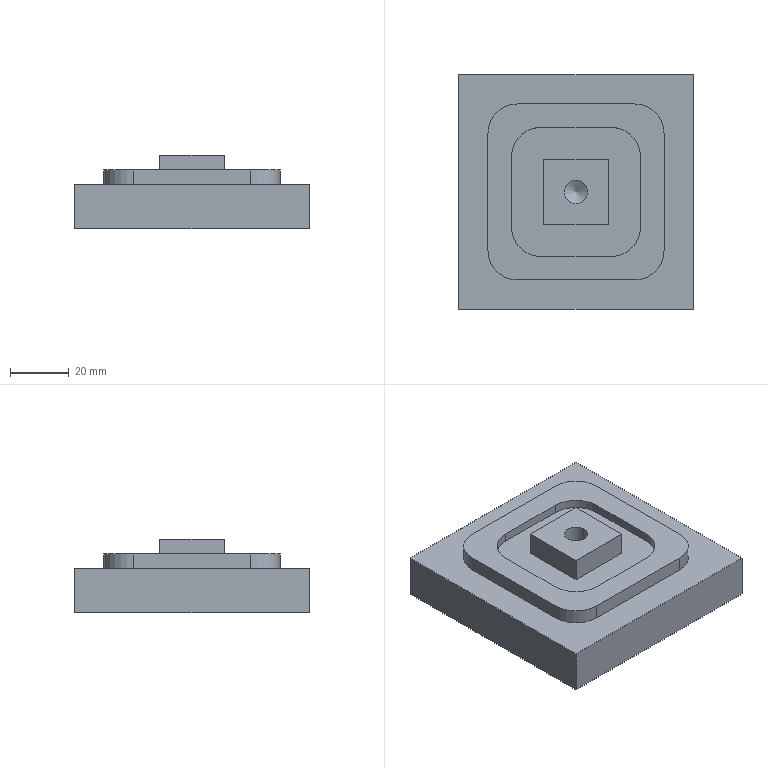NC program | NX | posted with a generic post | part box 80 x 80 x 25 mm
Whole program:
N10 G17 G21 G94 G90
(PLANAR_MILL , TOOL : T1D12)
N12 T01 M6
N14 G53
N16 G17 G0 G90 X32.505 Y-52. S2000 M3
N18 G43 Z10. H1
N20 Z2.
N22 G94 G1 Z-1. F1500.
N24 Y-40.
N26 X-40.
N28 Y-32.21
N30 X-32.8
N32 G3 X-32.21 Y-32.8 R17.69
N34 G1 X-32.8
N36 Y-32.21
N38 X-40.
N40 Y40.
N42 X-32.21
N44 Y32.8
N46 G3 X-32.8 Y32.21 R17.69
N48 G1 Y32.8
N50 X-32.21
N52 Y40.
N54 X40.
N56 Y32.21
N58 X32.8
N60 G3 X32.21 Y32.8 R17.69
N62 G1 X32.8
N64 Y32.21
N66 X40.
N68 Y-40.
N70 X32.505
N72 Y-32.8
N74 X32.21
N76 G3 X32.8 Y-32.21 R17.69
N78 G1 X31.758 Y-31.217
N80 G2 X20. Y-36.25 R16.25
N82 G1 X-20.
N84 G2 X-36.25 Y-20. R16.25
N86 G1 Y20.
N88 G2 X-20. Y36.25 R16.25
N90 G1 X20.
N92 G2 X36.25 Y20. R16.25
N94 G1 Y-20.
N96 G2 X31.758 Y-31.217 R16.25
N98 G1 X32.8 Y-32.21
N100 Y-32.8
N102 X32.505
N104 Y-52.
N106 Z2.
N108 G0 Z1.
N110 G1 Z-2.
N112 Y-40.
N114 X-40.
N116 Y-32.21
N118 X-32.8
N120 G3 X-32.21 Y-32.8 R17.69
N122 G1 X-32.8
N124 Y-32.21
N126 X-40.
N128 Y40.
N130 X-32.21
N132 Y32.8
N134 G3 X-32.8 Y32.21 R17.69
N136 G1 Y32.8
N138 X-32.21
N140 Y40.
N142 X40.
N144 Y32.21
N146 X32.8
N148 G3 X32.21 Y32.8 R17.69
N150 G1 X32.8
N152 Y32.21
N154 X40.
N156 Y-40.
N158 X32.505
N160 Y-32.8
N162 X32.21
N164 G3 X32.8 Y-32.21 R17.69
N166 G1 X31.758 Y-31.217
N168 G2 X20. Y-36.25 R16.25
N170 G1 X-20.
N172 G2 X-36.25 Y-20. R16.25
N174 G1 Y20.
N176 G2 X-20. Y36.25 R16.25
N178 G1 X20.
N180 G2 X36.25 Y20. R16.25
N182 G1 Y-20.
N184 G2 X31.758 Y-31.217 R16.25
N186 G1 X32.8 Y-32.21
N188 Y-32.8
N190 X32.505
N192 Y-52.
N194 Z1.
N196 G0 Z0.
N198 G1 Z-3.
N200 Y-40.
N202 X-40.
N204 Y-32.21
N206 X-32.8
N208 G3 X-32.21 Y-32.8 R17.69
N210 G1 X-32.8
N212 Y-32.21
N214 X-40.
N216 Y40.
N218 X-32.21
N220 Y32.8
N222 G3 X-32.8 Y32.21 R17.69
N224 G1 Y32.8
N226 X-32.21
N228 Y40.
N230 X40.
N232 Y32.21
N234 X32.8
N236 G3 X32.21 Y32.8 R17.69
N238 G1 X32.8
N240 Y32.21
N242 X40.
N244 Y-40.
N246 X32.505
N248 Y-32.8
N250 X32.21
N252 G3 X32.8 Y-32.21 R17.69
N254 G1 X31.758 Y-31.217
N256 G2 X20. Y-36.25 R16.25
N258 G1 X-20.
N260 G2 X-36.25 Y-20. R16.25
N262 G1 Y20.
N264 G2 X-20. Y36.25 R16.25
N266 G1 X20.
N268 G2 X36.25 Y20. R16.25
N270 G1 Y-20.
N272 G2 X31.758 Y-31.217 R16.25
N274 G1 X32.8 Y-32.21
N276 Y-32.8
N278 X32.505
N280 Y-52.
N282 Z0.
N284 G0 Z-1.
N286 G1 Z-4.
N288 Y-40.
N290 X-40.
N292 Y-32.21
N294 X-32.8
N296 G3 X-32.21 Y-32.8 R17.69
N298 G1 X-32.8
N300 Y-32.21
N302 X-40.
N304 Y40.
N306 X-32.21
N308 Y32.8
N310 G3 X-32.8 Y32.21 R17.69
N312 G1 Y32.8
N314 X-32.21
N316 Y40.
N318 X40.
N320 Y32.21
N322 X32.8
N324 G3 X32.21 Y32.8 R17.69
N326 G1 X32.8
N328 Y32.21
N330 X40.
N332 Y-40.
N334 X32.505
N336 Y-32.8
N338 X32.21
N340 G3 X32.8 Y-32.21 R17.69
N342 G1 X31.758 Y-31.217
N344 G2 X20. Y-36.25 R16.25
N346 G1 X-20.
N348 G2 X-36.25 Y-20. R16.25
N350 G1 Y20.
N352 G2 X-20. Y36.25 R16.25
N354 G1 X20.
N356 G2 X36.25 Y20. R16.25
N358 G1 Y-20.
N360 G2 X31.758 Y-31.217 R16.25
N362 G1 X32.8 Y-32.21
N364 Y-32.8
N366 X32.505
N368 Y-52.
N370 Z-1.
N372 G0 Z-2.
N374 G1 Z-5.
N376 Y-40.
N378 X-40.
N380 Y-32.21
N382 X-32.8
N384 G3 X-32.21 Y-32.8 R17.69
N386 G1 X-32.8
N388 Y-32.21
N390 X-40.
N392 Y40.
N394 X-32.21
N396 Y32.8
N398 G3 X-32.8 Y32.21 R17.69
N400 G1 Y32.8
N402 X-32.21
N404 Y40.
N406 X40.
N408 Y32.21
N410 X32.8
N412 G3 X32.21 Y32.8 R17.69
N414 G1 X32.8
N416 Y32.21
N418 X40.
N420 Y-40.
N422 X32.505
N424 Y-32.8
N426 X32.21
N428 G3 X32.8 Y-32.21 R17.69
N430 G1 X31.758 Y-31.217
N432 G2 X20. Y-36.25 R16.25
N434 G1 X-20.
N436 G2 X-36.25 Y-20. R16.25
N438 G1 Y20.
N440 G2 X-20. Y36.25 R16.25
N442 G1 X20.
N444 G2 X36.25 Y20. R16.25
N446 G1 Y-20.
N448 G2 X31.758 Y-31.217 R16.25
N450 G1 X32.8 Y-32.21
N452 Y-32.8
N454 X32.505
N456 Y-52.
N458 Z-2.
N460 G0 Z-3.
N462 G1 Z-6.
N464 Y-40.
N466 X-40.
N468 Y-32.21
N470 X-32.8
N472 G3 X-32.21 Y-32.8 R17.69
N474 G1 X-32.8
N476 Y-32.21
N478 X-40.
N480 Y40.
N482 X-32.21
N484 Y32.8
N486 G3 X-32.8 Y32.21 R17.69
N488 G1 Y32.8
N490 X-32.21
N492 Y40.
N494 X40.
N496 Y32.21
N498 X32.8
N500 G3 X32.21 Y32.8 R17.69
N502 G1 X32.8
N504 Y32.21
N506 X40.
N508 Y-40.
N510 X32.505
N512 Y-32.8
N514 X32.21
N516 G3 X32.8 Y-32.21 R17.69
N518 G1 X31.758 Y-31.217
N520 G2 X20. Y-36.25 R16.25
N522 G1 X-20.
N524 G2 X-36.25 Y-20. R16.25
N526 G1 Y20.
N528 G2 X-20. Y36.25 R16.25
N530 G1 X20.
N532 G2 X36.25 Y20. R16.25
N534 G1 Y-20.
N536 G2 X31.758 Y-31.217 R16.25
N538 G1 X32.8 Y-32.21
N540 Y-32.8
N542 X32.505
N544 Y-52.
N546 Z-3.
N548 G0 Z-4.
N550 G1 Z-7.
N552 Y-40.
N554 X-40.
N556 Y-32.21
N558 X-32.8
N560 G3 X-32.21 Y-32.8 R17.69
N562 G1 X-32.8
N564 Y-32.21
N566 X-40.
N568 Y40.
N570 X-32.21
N572 Y32.8
N574 G3 X-32.8 Y32.21 R17.69
N576 G1 Y32.8
N578 X-32.21
N580 Y40.
N582 X40.
N584 Y32.21
N586 X32.8
N588 G3 X32.21 Y32.8 R17.69
N590 G1 X32.8
N592 Y32.21
N594 X40.
N596 Y-40.
N598 X32.505
N600 Y-32.8
N602 X32.21
N604 G3 X32.8 Y-32.21 R17.69
N606 G1 X31.758 Y-31.217
N608 G2 X20. Y-36.25 R16.25
N610 G1 X-20.
N612 G2 X-36.25 Y-20. R16.25
N614 G1 Y20.
N616 G2 X-20. Y36.25 R16.25
N618 G1 X20.
N620 G2 X36.25 Y20. R16.25
N622 G1 Y-20.
N624 G2 X31.758 Y-31.217 R16.25
N626 G1 X32.8 Y-32.21
N628 Y-32.8
N630 X32.505
N632 Y-52.
N634 Z-4.
N636 G0 Z-5.
N638 G1 Z-8.
N640 Y-40.
N642 X-40.
N644 Y-32.21
N646 X-32.8
N648 G3 X-32.21 Y-32.8 R17.69
N650 G1 X-32.8
N652 Y-32.21
N654 X-40.
N656 Y40.
N658 X-32.21
N660 Y32.8
N662 G3 X-32.8 Y32.21 R17.69
N664 G1 Y32.8
N666 X-32.21
N668 Y40.
N670 X40.
N672 Y32.21
N674 X32.8
N676 G3 X32.21 Y32.8 R17.69
N678 G1 X32.8
N680 Y32.21
N682 X40.
N684 Y-40.
N686 X32.505
N688 Y-32.8
N690 X32.21
N692 G3 X32.8 Y-32.21 R17.69
N694 G1 X31.758 Y-31.217
N696 G2 X20. Y-36.25 R16.25
N698 G1 X-20.
N700 G2 X-36.25 Y-20. R16.25
N702 G1 Y20.
N704 G2 X-20. Y36.25 R16.25
N706 G1 X20.
N708 G2 X36.25 Y20. R16.25
N710 G1 Y-20.
N712 G2 X31.758 Y-31.217 R16.25
N714 G1 X32.8 Y-32.21
N716 Y-32.8
N718 X32.505
N720 Y-52.
N722 Z-5.
N724 G0 Z-6.
N726 G1 Z-9.
N728 Y-40.
N730 X-40.
N732 Y-32.21
N734 X-32.8
N736 G3 X-32.21 Y-32.8 R17.69
N738 G1 X-32.8
N740 Y-32.21
N742 X-40.
N744 Y40.
N746 X-32.21
N748 Y32.8
N750 G3 X-32.8 Y32.21 R17.69
N752 G1 Y32.8
N754 X-32.21
N756 Y40.
N758 X40.
N760 Y32.21
N762 X32.8
N764 G3 X32.21 Y32.8 R17.69
N766 G1 X32.8
N768 Y32.21
N770 X40.
N772 Y-40.
N774 X32.505
N776 Y-32.8
N778 X32.21
N780 G3 X32.8 Y-32.21 R17.69
N782 G1 X31.758 Y-31.217
N784 G2 X20. Y-36.25 R16.25
N786 G1 X-20.
N788 G2 X-36.25 Y-20. R16.25
N790 G1 Y20.
N792 G2 X-20. Y36.25 R16.25
N794 G1 X20.
N796 G2 X36.25 Y20. R16.25
N798 G1 Y-20.
N800 G2 X31.758 Y-31.217 R16.25
N802 G1 X32.8 Y-32.21
N804 Y-32.8
N806 X32.505
N808 Y-52.
N810 Z-6.
N812 G0 Z-6.85
N814 G1 Z-9.85
N816 Y-40.
N818 X-40.
N820 Y-32.21
N822 X-32.8
N824 G3 X-32.21 Y-32.8 R17.69
N826 G1 X-32.8
N828 Y-32.21
N830 X-40.
N832 Y40.
N834 X-32.21
N836 Y32.8
N838 G3 X-32.8 Y32.21 R17.69
N840 G1 Y32.8
N842 X-32.21
N844 Y40.
N846 X40.
N848 Y32.21
N850 X32.8
N852 G3 X32.21 Y32.8 R17.69
N854 G1 X32.8
N856 Y32.21
N858 X40.
N860 Y-40.
N862 X32.505
N864 Y-32.8
N866 X32.21
N868 G3 X32.8 Y-32.21 R17.69
N870 G1 X31.758 Y-31.217
N872 G2 X20. Y-36.25 R16.25
N874 G1 X-20.
N876 G2 X-36.25 Y-20. R16.25
N878 G1 Y20.
N880 G2 X-20. Y36.25 R16.25
N882 G1 X20.
N884 G2 X36.25 Y20. R16.25
N886 G1 Y-20.
N888 G2 X31.758 Y-31.217 R16.25
N890 G1 X32.8 Y-32.21
N892 Y-32.8
N894 X32.505
N896 Y-52.
N898 Z-6.85
N900 G0 Z10.
(PLANAR_MILL_1 , TOOL : T1D12)
N902 X-42. Y0. S1500
N904 Z0.
N906 G1 Z-1. F1200.
N908 X-30.
N910 Y20.
N912 G2 X-20. Y30. R10.
N914 G1 X20.
N916 G2 X30. Y20. R10.
N918 G1 Y-20.
N920 G2 X20. Y-30. R10.
N922 G1 X-20.
N924 G2 X-30. Y-20. R10.
N926 G1 Y0.
N928 X-21.6
N930 Y20.
N932 G2 X-20. Y21.6 R1.6
N934 G1 X20.
N936 G2 X21.6 Y20. R1.6
N938 G1 Y-20.
N940 G2 X20.001 Y-21.6 R1.6
N942 G1 X-20.
N944 G2 X-21.6 Y-20. R1.6
N946 G1 Y0.
N948 X-17.25
N950 Y11.
N952 G2 X-11. Y17.25 R6.25
N954 G1 X11.
N956 G2 X17.25 Y11. R6.25
N958 G1 Y-11.
N960 G2 X11. Y-17.25 R6.25
N962 G1 X-11.
N964 G2 X-17.25 Y-11. R6.25
N966 G1 Y0.
N968 Z0.
N970 G0 X-42. Z-1.
N972 G1 Z-2.
N974 X-30.
N976 Y20.
N978 G2 X-20. Y30. R10.
N980 G1 X20.
N982 G2 X30. Y20. R10.
N984 G1 Y-20.
N986 G2 X20. Y-30. R10.
N988 G1 X-20.
N990 G2 X-30. Y-20. R10.
N992 G1 Y0.
N994 X-21.6
N996 Y20.
N998 G2 X-20. Y21.6 R1.6
N1000 G1 X20.
N1002 G2 X21.6 Y20. R1.6
N1004 G1 Y-20.
N1006 G2 X20.001 Y-21.6 R1.6
N1008 G1 X-20.
N1010 G2 X-21.6 Y-20. R1.6
N1012 G1 Y0.
N1014 X-17.25
N1016 Y11.
N1018 G2 X-11. Y17.25 R6.25
N1020 G1 X11.
N1022 G2 X17.25 Y11. R6.25
N1024 G1 Y-11.
N1026 G2 X11. Y-17.25 R6.25
N1028 G1 X-11.
N1030 G2 X-17.25 Y-11. R6.25
N1032 G1 Y0.
N1034 Z-1.
N1036 G0 X-42. Z-2.
N1038 G1 Z-3.
N1040 X-30.
N1042 Y20.
N1044 G2 X-20. Y30. R10.
N1046 G1 X20.
N1048 G2 X30. Y20. R10.
N1050 G1 Y-20.
N1052 G2 X20. Y-30. R10.
N1054 G1 X-20.
N1056 G2 X-30. Y-20. R10.
N1058 G1 Y0.
N1060 X-21.6
N1062 Y20.
N1064 G2 X-20. Y21.6 R1.6
N1066 G1 X20.
N1068 G2 X21.6 Y20. R1.6
N1070 G1 Y-20.
N1072 G2 X20.001 Y-21.6 R1.6
N1074 G1 X-20.
N1076 G2 X-21.6 Y-20. R1.6
N1078 G1 Y0.
N1080 X-17.25
N1082 Y11.
N1084 G2 X-11. Y17.25 R6.25
N1086 G1 X11.
N1088 G2 X17.25 Y11. R6.25
N1090 G1 Y-11.
N1092 G2 X11. Y-17.25 R6.25
N1094 G1 X-11.
N1096 G2 X-17.25 Y-11. R6.25
N1098 G1 Y0.
N1100 Z-2.
N1102 G0 X-42. Z-3.
N1104 G1 Z-4.
N1106 X-30.
N1108 Y20.
N1110 G2 X-20. Y30. R10.
N1112 G1 X20.
N1114 G2 X30. Y20. R10.
N1116 G1 Y-20.
N1118 G2 X20. Y-30. R10.
N1120 G1 X-20.
N1122 G2 X-30. Y-20. R10.
N1124 G1 Y0.
N1126 X-21.6
N1128 Y20.
N1130 G2 X-20. Y21.6 R1.6
N1132 G1 X20.
N1134 G2 X21.6 Y20. R1.6
N1136 G1 Y-20.
N1138 G2 X20.001 Y-21.6 R1.6
N1140 G1 X-20.
N1142 G2 X-21.6 Y-20. R1.6
N1144 G1 Y0.
N1146 X-17.25
N1148 Y11.
N1150 G2 X-11. Y17.25 R6.25
N1152 G1 X11.
N1154 G2 X17.25 Y11. R6.25
N1156 G1 Y-11.
N1158 G2 X11. Y-17.25 R6.25
N1160 G1 X-11.
N1162 G2 X-17.25 Y-11. R6.25
N1164 G1 Y0.
N1166 Z-3.
N1168 G0 X-42. Z-3.75
N1170 G1 Z-4.75
N1172 X-30.
N1174 Y20.
N1176 G2 X-20. Y30. R10.
N1178 G1 X20.
N1180 G2 X30. Y20. R10.
N1182 G1 Y-20.
N1184 G2 X20. Y-30. R10.
N1186 G1 X-20.
N1188 G2 X-30. Y-20. R10.
N1190 G1 Y0.
N1192 X-21.6
N1194 Y20.
N1196 G2 X-20. Y21.6 R1.6
N1198 G1 X20.
N1200 G2 X21.6 Y20. R1.6
N1202 G1 Y-20.
N1204 G2 X20.001 Y-21.6 R1.6
N1206 G1 X-20.
N1208 G2 X-21.6 Y-20. R1.6
N1210 G1 Y0.
N1212 X-17.25
N1214 Y11.
N1216 G2 X-11. Y17.25 R6.25
N1218 G1 X11.
N1220 G2 X17.25 Y11. R6.25
N1222 G1 Y-11.
N1224 G2 X11. Y-17.25 R6.25
N1226 G1 X-11.
N1228 G2 X-17.25 Y-11. R6.25
N1230 G1 Y0.
N1232 Z-3.75
N1234 G0 Z10.
N1236 M5
(PLANAR_MILL_2 , TOOL : T2D6)
N1238 T02 M6
N1240 G53
N1242 G17 G0 G90 X13.67 Y-12.994 S2000 M3
N1244 G43 Z10. H2
N1246 Z-2.
N1248 G94 G3 X13.67 Y-12.994 Z-3.319 I1.325 J-2.001 F1000.
N1250 X13.67 Y-12.994 Z-4.639 I1.325 J-2.001
N1252 X13.67 Y-12.994 Z-5.958 I1.325 J-2.001
N1254 X13.298 Y-13.298 Z-6. R2.4
N1256 G2 X11. Y-14.25 R3.25
N1258 G1 X-11.
N1260 G2 X-14.25 Y-11. R3.25
N1262 G1 Y11.
N1264 G2 X-11. Y14.25 R3.25
N1266 G1 X11.
N1268 G2 X14.25 Y11. R3.25
N1270 G1 Y-11.
N1272 G2 X13.298 Y-13.298 R3.25
N1274 G1 X14.652 Y-14.652
N1276 G3 X15.75 Y-12. R3.75
N1278 G1 Y12.
N1280 G3 X12. Y15.75 R3.75
N1282 G1 X-12.
N1284 G3 X-15.75 Y12. R3.75
N1286 G1 Y-12.
N1288 G3 X-12. Y-15.75 R3.75
N1290 G1 X12.001
N1292 G3 X14.652 Y-14.652 R3.75
N1294 G1 X16.773 Y-16.773
N1296 G3 X18.75 Y-12. R6.75
N1298 G1 Y12.
N1300 G3 X12. Y18.75 R6.75
N1302 G1 X-12.
N1304 G3 X-18.75 Y12. R6.75
N1306 G1 Y-12.
N1308 G3 X-12. Y-18.75 R6.75
N1310 G1 X12.
N1312 G3 X16.773 Y-16.773 R6.75
N1314 G1 Z-3.
N1316 G0 Z-2.
N1318 X13.67 Y-12.994
N1320 Z-3.
N1322 G3 X13.67 Y-12.994 Z-4.319 I1.325 J-2.001
N1324 X13.67 Y-12.994 Z-5.639 I1.325 J-2.001
N1326 X13.67 Y-12.994 Z-6.958 I1.325 J-2.001
N1328 X13.298 Y-13.298 Z-7. R2.4
N1330 G2 X11. Y-14.25 R3.25
N1332 G1 X-11.
N1334 G2 X-14.25 Y-11. R3.25
N1336 G1 Y11.
N1338 G2 X-11. Y14.25 R3.25
N1340 G1 X11.
N1342 G2 X14.25 Y11. R3.25
N1344 G1 Y-11.
N1346 G2 X13.298 Y-13.298 R3.25
N1348 G1 X14.652 Y-14.652
N1350 G3 X15.75 Y-12. R3.75
N1352 G1 Y12.
N1354 G3 X12. Y15.75 R3.75
N1356 G1 X-12.
N1358 G3 X-15.75 Y12. R3.75
N1360 G1 Y-12.
N1362 G3 X-12. Y-15.75 R3.75
N1364 G1 X12.001
N1366 G3 X14.652 Y-14.652 R3.75
N1368 G1 X16.773 Y-16.773
N1370 G3 X18.75 Y-12. R6.75
N1372 G1 Y12.
N1374 G3 X12. Y18.75 R6.75
N1376 G1 X-12.
N1378 G3 X-18.75 Y12. R6.75
N1380 G1 Y-12.
N1382 G3 X-12. Y-18.75 R6.75
N1384 G1 X12.
N1386 G3 X16.773 Y-16.773 R6.75
N1388 G1 Z-4.
N1390 G0 Z-3.
N1392 X12.645 Y-15.483
N1394 Z-4.
N1396 G3 X12.645 Y-15.483 Z-5.319 I2.35 J0.488
N1398 X12.645 Y-15.483 Z-6.639 I2.35 J0.488
N1400 X13.298 Y-13.298 Z-7.75 R-2.4
N1402 G2 X11. Y-14.25 R3.25
N1404 G1 X-11.
N1406 G2 X-14.25 Y-11. R3.25
N1408 G1 Y11.
N1410 G2 X-11. Y14.25 R3.25
N1412 G1 X11.
N1414 G2 X14.25 Y11. R3.25
N1416 G1 Y-11.
N1418 G2 X13.298 Y-13.298 R3.25
N1420 G1 X14.652 Y-14.652
N1422 G3 X15.75 Y-12. R3.75
N1424 G1 Y12.
N1426 G3 X12. Y15.75 R3.75
N1428 G1 X-12.
N1430 G3 X-15.75 Y12. R3.75
N1432 G1 Y-12.
N1434 G3 X-12. Y-15.75 R3.75
N1436 G1 X12.001
N1438 G3 X14.652 Y-14.652 R3.75
N1440 G1 X16.773 Y-16.773
N1442 G3 X18.75 Y-12. R6.75
N1444 G1 Y12.
N1446 G3 X12. Y18.75 R6.75
N1448 G1 X-12.
N1450 G3 X-18.75 Y12. R6.75
N1452 G1 Y-12.
N1454 G3 X-12. Y-18.75 R6.75
N1456 G1 X12.
N1458 G3 X16.773 Y-16.773 R6.75
N1460 G1 Z-4.75
N1462 G0 Z10.
N1464 M5
(PLANAR_MILL_COPY , TOOL : T1D12)
N1466 T01 M6
N1468 G53
N1470 G17 G0 G90 X-52. Y32.496 S80 M3
N1472 G43 Z10. H1
N1474 Z-7.
N1476 G94 G1 Z-10. F100.
N1478 X-40.
N1480 Y40.
N1482 X40.
N1484 Y30.993
N1486 X34.
N1488 G3 X30.993 Y34. R17.8
N1490 G1 X34.
N1492 Y30.993
N1494 X40.
N1496 Y-40.
N1498 X30.993
N1500 Y-34.
N1502 G3 X34. Y-30.993 R17.8
N1504 G1 Y-34.
N1506 X30.993
N1508 Y-40.
N1510 X-40.
N1512 Y-30.993
N1514 X-34.
N1516 G3 X-30.993 Y-34. R17.8
N1518 G1 X-34.
N1520 Y-30.993
N1522 X-40.
N1524 Y32.496
N1526 X-34.
N1528 Y34.
N1530 X-30.993
N1532 G3 X-34. Y30.993 R17.8
N1534 G1 X-33.056 Y30.252
N1536 G2 X-20. Y36.6 R16.6
N1538 G1 X20.
N1540 G2 X36.6 Y20. R16.6
N1542 G1 Y-20.
N1544 G2 X20. Y-36.6 R16.6
N1546 G1 X-20.
N1548 G2 X-36.6 Y-20. R16.6
N1550 G1 Y20.
N1552 G2 X-33.056 Y30.252 R16.6
N1554 G1 X-34. Y30.993
N1556 Y32.496
N1558 X-36.86 Y35.05
N1560 X-31.937 Y30.655
N1562 G2 X-20. Y36. R16.
N1564 G1 X20.
N1566 G2 X36. Y20. R16.
N1568 G1 Y-20.
N1570 G2 X20. Y-36. R16.
N1572 G1 X-20.
N1574 G2 X-36. Y-20. R16.
N1576 G1 Y20.
N1578 G2 X-31.937 Y30.655 R16.
N1580 G1 X-36.413 Y34.65
N1582 Z-7.
N1584 G0 Z10.
(PLANAR_MILL_1_COPY , TOOL : T1D12)
N1586 X-42. Y-18.713 S1500
N1588 Z-4.
N1590 G1 Z-5. F1200.
N1592 X-30.
N1594 Y20.
N1596 G2 X-20. Y30. R10.
N1598 G1 X20.
N1600 G2 X30. Y20. R10.
N1602 G1 Y-20.
N1604 G2 X20. Y-30. R10.
N1606 G1 X-20.
N1608 G2 X-30. Y-20. R10.
N1610 G1 Y-18.713
N1612 X-25.2
N1614 Y20.
N1616 G2 X-20. Y25.2 R5.2
N1618 G1 X-17.426
N1620 Y20.4
N1622 G3 X-20.4 Y17.426 R10.
N1624 G1 Y20.
N1626 G2 X-20. Y20.4 R0.4
N1628 G1 X-17.426
N1630 Y25.2
N1632 X20.
N1634 G2 X25.2 Y20. R5.2
N1636 G1 Y17.426
N1638 X20.4
N1640 G3 X17.426 Y20.4 R10.
N1642 G1 X20.
N1644 G2 X20.4 Y20. R0.4
N1646 G1 Y17.426
N1648 X25.2
N1650 Y-20.
N1652 G2 X20.001 Y-25.2 R5.2
N1654 G1 X17.426
N1656 Y-20.4
N1658 G3 X20.4 Y-17.426 R10.
N1660 G1 Y-20.
N1662 G2 X20. Y-20.4 R0.4
N1664 G1 X17.426
N1666 Y-25.2
N1668 X-20.
N1670 G2 X-25.2 Y-20. R5.2
N1672 G1 Y-18.713
N1674 X-20.4
N1676 Y-17.426
N1678 G3 X-17.426 Y-20.4 R10.
N1680 G1 X-20.
N1682 G2 X-20.4 Y-20. R0.4
N1684 G1 Y-18.713
N1686 X-42.
N1688 Z-4.
N1690 G0 Z10.
N1692 M5
(PLANAR_MILL_2_COPY , TOOL : T2D6)
N1694 T02 M6
N1696 G53
N1698 G17 G0 G90 X16.149 Y-17.154 S100 M3
N1700 G43 Z10. H2
N1702 Z-2.
N1704 G94 G3 X16.149 Y-17.154 Z-3.319 I-1.118 J2.124 F200.
N1706 X16.149 Y-17.154 Z-4.639 I-1.118 J2.124
N1708 X16.149 Y-17.154 Z-5.958 I-1.118 J2.124
N1710 X16.149 Y-17.154 Z-7.277 I-1.118 J2.124
N1712 X13.333 Y-13.333 Z-8. R-2.4
N1714 G2 X11. Y-14.3 R3.3
N1716 G1 X-11.
N1718 G2 X-14.3 Y-11. R3.3
N1720 G1 Y11.
N1722 G2 X-11. Y14.3 R3.3
N1724 G1 X11.
N1726 G2 X14.3 Y11. R3.3
N1728 G1 Y-11.
N1730 G2 X13.333 Y-13.333 R3.3
N1732 G1 X14.616 Y-14.616
N1734 G3 X15.7 Y-12. R3.7
N1736 G1 Y12.
N1738 G3 X12. Y15.7 R3.7
N1740 G1 X-12.
N1742 G3 X-15.7 Y12. R3.7
N1744 G1 Y-12.
N1746 G3 X-12. Y-15.7 R3.7
N1748 G1 X12.001
N1750 G3 X14.616 Y-14.616 R3.7
N1752 G1 X16.738 Y-16.738
N1754 G3 X18.7 Y-12. R6.7
N1756 G1 Y12.
N1758 G3 X12. Y18.7 R6.7
N1760 G1 X-12.
N1762 G3 X-18.7 Y12. R6.7
N1764 G1 Y-12.
N1766 G3 X-12. Y-18.7 R6.7
N1768 G1 X12.
N1770 G3 X16.738 Y-16.738 R6.7
N1772 G1 Z-5.
N1774 G0 Z-2.
N1776 X0.949 Y-18.729
N1778 G3 X0.949 Y-18.729 Z-3.352 I-0.949 J2.269
N1780 X0.949 Y-18.729 Z-4.705 I-0.949 J2.269
N1782 X0.949 Y-18.729 Z-6.057 I-0.949 J2.269
N1784 X0.949 Y-18.729 Z-7.409 I-0.949 J2.269
N1786 X0. Y-14. Z-8. R2.46
N1788 G1 X-11.
N1790 G2 X-14. Y-11. R3.
N1792 G1 Y11.
N1794 G2 X-11. Y14. R3.
N1796 G1 X11.
N1798 G2 X14. Y11. R3.
N1800 G1 Y-11.
N1802 G2 X11. Y-14. R3.
N1804 G1 X0.
N1806 Z-5.
N1808 G0 Z-2.
N1810 X-0.949 Y-14.271
N1812 G3 X-0.949 Y-14.271 Z-3.352 I0.949 J-2.269
N1814 X-0.949 Y-14.271 Z-4.705 I0.949 J-2.269
N1816 X-0.949 Y-14.271 Z-6.057 I0.949 J-2.269
N1818 X-0.949 Y-14.271 Z-7.409 I0.949 J-2.269
N1820 X0. Y-19. Z-8. R2.46
N1822 G1 X12.
N1824 G3 X19. Y-12. R7.
N1826 G1 Y12.
N1828 G3 X12. Y19. R7.
N1830 G1 X-12.
N1832 G3 X-19. Y12. R7.
N1834 G1 Y-12.
N1836 G3 X-12. Y-19. R7.
N1838 G1 X0.
N1840 Z-5.
N1842 G0 Z10.
N1844 M5
(SPOT_DRILLING , TOOL : SPOTDRILLING_TOOL_Z10)
N1846 T00 M6
N1848 G53
N1850 G17 G0 G90 X0. Y0. S0 M3
N1852 G43 Z10. H0
N1854 G94 G82 G99 Z-1. F200. P2000 R3.
N1856 G80
N1858 G0 X0. Y0. Z10.
N1860 M5
(DRILLING , TOOL : T3Z8)
N1862 T03 M6
N1864 G53
N1866 G17 G0 G90 X0. Y0. S100 M3
N1868 G43 Z10. H3
N1870 G94 G82 G99 Z-10.403 F85. P2000 R3.
N1872 G80
N1874 G0 X0. Y0. Z10.
N1876 M5
N1878 M2